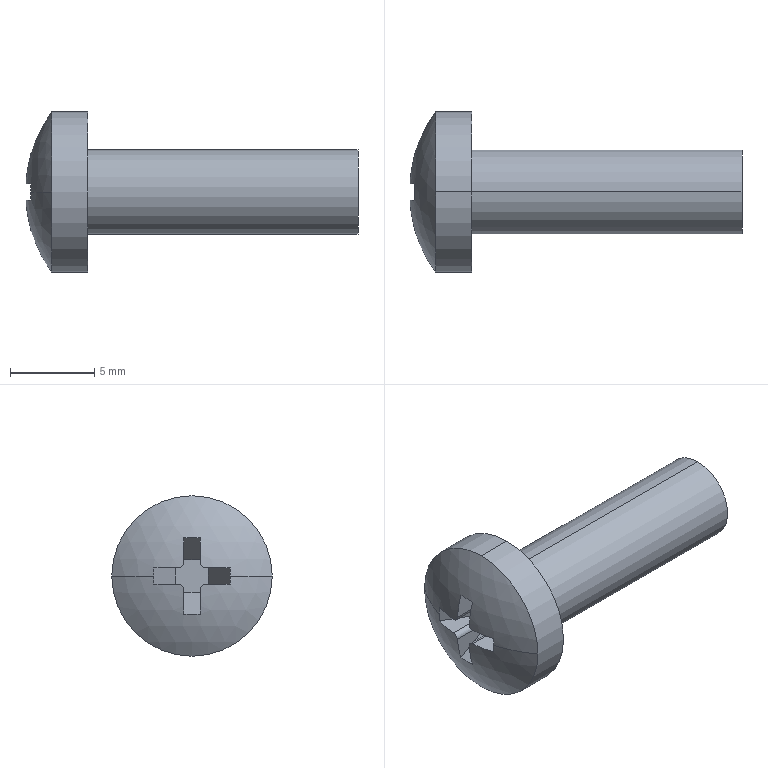Part | STEP file | cross recessed pan head screws gbV1.201001_GB_CROSS_SCREWS_TYPE1 M5X16-16  H type-N | 1 solid | 25 faces | box 19.658 x 9.5 x 9.5 mm | volume 509.153 mm3 | plane 15 | cylinder 8 | sphere 2 | commonest cylinder face diameters 0.6 x4 5 x2 9.5 x2